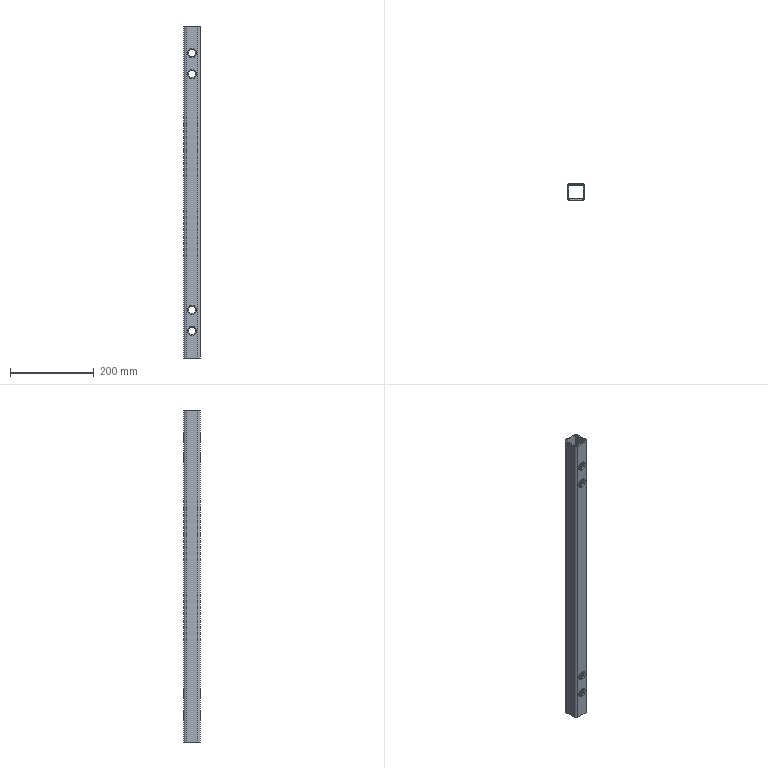Part | STEP file | IN-01-01-01-07 | 1 solid | 54 faces | box 40 x 40 x 795 mm | volume 317936 mm3 | cylinder 28 | cone 16 | plane 10 | commonest cylinder face diameters 17.5 x16 5.8 x4 10 x4 11.6 x4